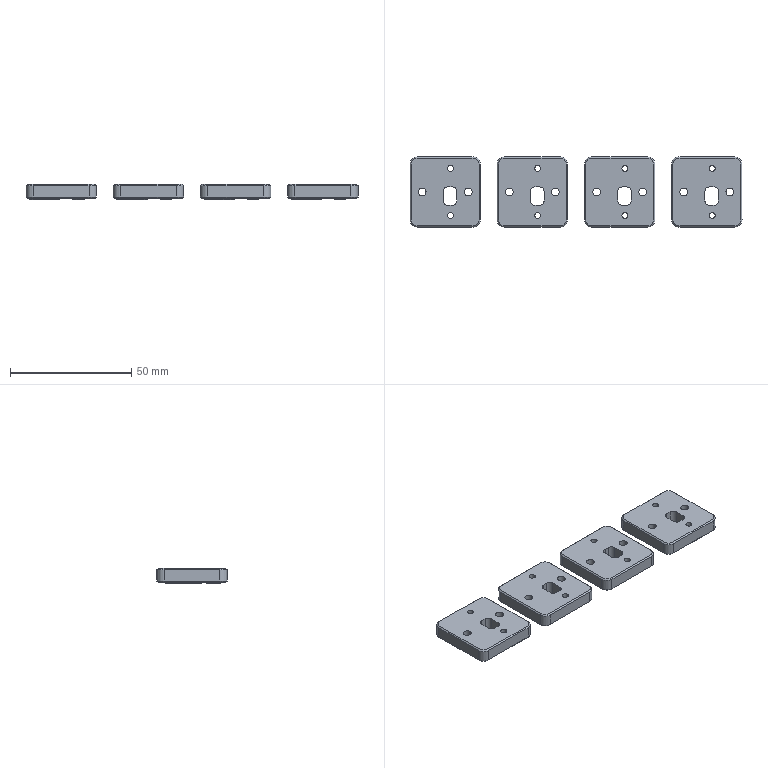NC program | NX | posted with a generic post | part box 137 x 29 x 6.3 mm
Lines 43 to 1179 of 3650:
(FLOOR_WALL_1 , TOOL : D2)
N84 T12 M6
N86 G54
N88 G17 G0 G90 X54. Y-16.497 S9500 M3
N90 G43 Z30. H12
N92 Z0.843
N94 G94 G1 Z-0.158 F1100.
N96 Y-14.497
N98 X39.503
N100 Y14.497
N102 X68.497
N104 Y-14.497
N106 X54.
N108 Y-13.497
N110 X40.503
N112 Y-10.866
N114 G3 X41.516 Y-11.2 R1.7
N116 G1 X45.516
N118 G3 X47.216 Y-9.5 R1.7
N120 G1 Y-8.5
N122 G3 X45.516 Y-6.8 R1.7
N124 G1 X41.508
N126 G3 X40.503 Y-7.134 R1.7
N128 G1 X40.622 Y-7.295
N130 G2 X41.516 Y-7. R1.5
N132 G1 X45.516
N134 G2 X47.016 Y-8.5 R1.5
N136 G1 Y-9.5
N138 G2 X45.516 Y-11. R1.5
N140 G1 X41.516
N142 G2 X40.016 Y-9.5 R1.5
N144 G1 Y-8.5
N146 G2 X40.622 Y-7.295 R1.5
N148 G1 X40.503 Y-7.134
N150 Y13.497
N152 X67.497
N154 Y-13.497
N156 X54.
N158 Y-12.497
N160 X41.503
N162 Y-12.2
N164 X45.516
N166 G3 X48.216 Y-9.5 R2.7
N168 G1 Y-8.5
N170 G3 X45.516 Y-5.8 R2.7
N172 G1 X42.503
N174 X41.503
N176 Y12.497
N178 X59.288
N180 G3 X62.317 Y12.497 R-3.2
N182 G1 X62.222 Y12.321
N184 G2 X63.445 Y8.258 R3.
N186 X62.222 Y12.321 R-3.
N188 G1 X62.317 Y12.497
N190 X66.497
N192 Y-12.497
N194 X54.
N196 Y-11.497
N198 X48.63
N200 G3 X49.216 Y-9.5 R3.7
N202 G1 Y-8.5
N204 G3 X49.206 Y-8.231 R3.7
N206 X48.3 Y-6. R-3.2
N208 G1 X48.301 Y-6.064
N210 X48.501 Y-6.06
N212 G2 X51.44 Y-3.001 R3.
N214 X48.501 Y-6.06 R-3.
N216 G1 X48.301 Y-6.064
N218 G3 X47.112 Y-5.162 R3.7
N220 G1 X47.543 Y-4.26
N222 G3 X47.726 Y-4.158 R3.45
N224 G1 X47.653 Y-4.314
N226 X47.543 Y-4.26
N228 X47.112 Y-5.162
N230 G3 X45.516 Y-4.8 R3.7
N232 G1 X42.503
N234 Y-3.632
N236 X43.503
N238 G3 X43.682 Y-3.8 R3.45
N240 G1 X43.503
N242 Y-3.632
N244 X42.503
N246 Y11.497
N248 X57.017
N250 G3 X64.588 Y11.497 R-4.2
N252 G1 X65.497
N254 Y-11.497
N256 X63.639
N258 G3 X59.364 Y-11.497 R-3.2
N260 G1 X59.498 Y-11.348
N262 G2 X59.269 Y-7.112 R3.
N264 X59.498 Y-11.348 R-3.
N266 G1 X59.364 Y-11.497
N268 X54.
N270 Y-10.497
N272 X50.109
N274 G3 X50.19 Y-9.99 R4.7
N276 X49.133 Y-2.531 R-4.2
N278 X47.248 Y1.997 R3.45
N280 X44.941 Y0.088 R1.7
N282 G2 X44.496 Y-0.45 R0.45
N284 G3 X43.557 Y-0.722 R1.7
N286 G1 X43.503 Y-0.759
N288 X43.618 Y-0.922
N290 G2 X44.494 Y-0.65 R1.5
N292 G3 X45.137 Y0.127 R0.65
N294 G2 X47.173 Y1.811 R1.5
N296 X43.221 Y-2.964 R-3.25
N298 X43.618 Y-0.922 R1.5
N300 G1 X43.503 Y-0.759
N302 Y10.497
N304 X55.667
N306 G3 X64.497 Y6.019 R5.2
N308 G1 Y-6.172
N310 G3 X57.535 Y-10.497 R4.2
N312 G1 X54.
N314 X55.349 Y-9.497
N316 G3 X50.391 Y-0.92 R5.2
N318 X50.197 Y0.128 R4.45
N320 X51.602 Y-0.614 R1.7
N322 G1 X52.7
N324 G3 X54.4 Y1.086 R1.7
N326 G1 Y3.227
N328 G3 X52.7 Y4.927 R1.7
N330 G1 X51.602
N332 G3 X49.902 Y3.227 R1.7
N334 G1 Y1.086
N336 G3 X49.926 Y0.798 R1.7
N338 G1 X50.123 Y0.832
N340 G2 X50.102 Y1.086 R1.5
N342 G1 Y3.227
N344 G2 X51.602 Y4.727 R1.5
N346 G1 X52.7
N348 G2 X54.2 Y3.227 R1.5
N350 G1 Y1.086
N352 G2 X52.7 Y-0.414 R1.5
N354 G1 X51.602
N356 G2 X50.123 Y0.832 R1.5
N358 G1 X49.926 Y0.798
N360 G3 X47.624 Y2.923 R4.45
N362 X44.503 Y2.112 R2.7
N364 G1 Y9.497
N366 X46.123
N368 G3 X45.8 Y8.5 R1.7
N370 G1 Y6.5
N372 G3 X46.716 Y4.992 R1.7
N374 G1 X46.254 Y4.105
N376 G3 X45.503 Y3.953 R3.7
N378 G1 Y4.683
N380 G3 X46.254 Y4.105 R2.7
N382 G1 X46.716 Y4.992
N384 G3 X47.5 Y4.8 R1.7
N386 G1 X48.963
N388 Y3.8
N390 G3 X48.906 Y3.379 R2.7
N392 X48.119 Y3.8 R5.45
N394 G1 X48.963
N396 Y4.8
N398 X50.5
N400 G3 X52.2 Y6.5 R1.7
N402 G1 Y8.5
N404 G3 X51.877 Y9.497 R1.7
N406 G1 X51.715 Y9.38
N408 G2 X52. Y8.5 R1.5
N410 G1 Y6.5
N412 G2 X50.5 Y5. R1.5
N414 G1 X47.5
N416 G2 X46. Y6.5 R1.5
N418 G1 Y8.5
N420 G2 X47.5 Y10. R1.5
N422 G1 X50.5
N424 G2 X51.715 Y9.38 R1.5
N426 G1 X51.877 Y9.497
N428 X54.605
N430 G3 X63.497 Y4.094 R6.2
N432 G1 Y-4.314
N434 G3 X58.135 Y-5.153 R5.2
N436 G1 X57.487 Y-4.391
N438 G3 X54.722 Y-0.703 R6.2
N440 X55.4 Y1.086 R2.7
N442 G1 Y3.227
N444 G3 X53.131 Y5.892 R2.7
N446 X53.2 Y6.5 R2.7
N448 G1 Y8.497
N450 X53.7
N452 G3 X62.497 Y2.68 R7.2
N454 G1 Y-2.996
N456 G3 X57.487 Y-4.391 R6.2
N458 G1 X57.97 Y-2.841
N460 G3 X56.072 Y-0.438 R7.2
N462 X56.272 Y0.12 R3.7
N464 X56.4 Y1.13 R3.7
N466 G1 Y2.76
N468 G3 X61.497 Y1.507 R8.2
N470 G1 Y-1.916
N472 G3 X57.97 Y-2.841 R7.2
N474 G1 X58.377 Y-1.534
N476 G3 X57.237 Y-0.141 R8.2
N478 X57.4 Y1.13 R4.7
N480 X60.497 Y0.483 R9.2
N482 G1 Y-0.978
N484 G3 X58.377 Y-1.534 R8.2
N486 G1 X58.75 Y-0.337
N488 X58.729 Y-0.309
N490 X58.796 Y-0.323
N492 X58.75 Y-0.337
N494 X57.487 Y-4.391
N496 X58.135 Y-5.153
N498 G3 X56.316 Y-9.497 R5.2
N500 G1 X55.349
N502 Y-10.497
N504 Z0.843
N506 G0 X54. Y-16.497 Z0.705
N508 G1 Z-0.295
N510 Y-14.497
N512 X39.503
N514 Y14.497
N516 X68.497
N518 Y-14.497
N520 X54.
N522 Y-13.497
N524 X40.503
N526 Y-10.866
N528 G3 X41.516 Y-11.2 R1.7
N530 G1 X45.516
N532 G3 X47.216 Y-9.5 R1.7
N534 G1 Y-8.5
N536 G3 X45.516 Y-6.8 R1.7
N538 G1 X41.508
N540 G3 X40.503 Y-7.134 R1.7
N542 G1 X40.622 Y-7.295
N544 G2 X41.516 Y-7. R1.5
N546 G1 X45.516
N548 G2 X47.016 Y-8.5 R1.5
N550 G1 Y-9.5
N552 G2 X45.516 Y-11. R1.5
N554 G1 X41.516
N556 G2 X40.016 Y-9.5 R1.5
N558 G1 Y-8.5
N560 G2 X40.622 Y-7.295 R1.5
N562 G1 X40.503 Y-7.134
N564 Y13.497
N566 X67.497
N568 Y-13.497
N570 X54.
N572 Y-12.497
N574 X41.503
N576 Y-12.2
N578 X45.516
N580 G3 X48.216 Y-9.5 R2.7
N582 G1 Y-8.5
N584 G3 X45.516 Y-5.8 R2.7
N586 G1 X42.503
N588 X41.503
N590 Y12.497
N592 X59.288
N594 G3 X62.317 Y12.497 R-3.2
N596 G1 X62.222 Y12.321
N598 G2 X63.445 Y8.258 R3.
N600 X62.222 Y12.321 R-3.
N602 G1 X62.317 Y12.497
N604 X66.497
N606 Y-12.497
N608 X54.
N610 Y-11.497
N612 X48.63
N614 G3 X49.216 Y-9.5 R3.7
N616 G1 Y-8.5
N618 G3 X49.206 Y-8.231 R3.7
N620 X48.3 Y-6. R-3.2
N622 G1 X48.301 Y-6.064
N624 X48.501 Y-6.06
N626 G2 X51.44 Y-3.001 R3.
N628 X48.501 Y-6.06 R-3.
N630 G1 X48.301 Y-6.064
N632 G3 X47.112 Y-5.162 R3.7
N634 G1 X47.543 Y-4.26
N636 G3 X47.726 Y-4.158 R3.45
N638 G1 X47.653 Y-4.314
N640 X47.543 Y-4.26
N642 X47.112 Y-5.162
N644 G3 X45.516 Y-4.8 R3.7
N646 G1 X42.503
N648 Y-3.632
N650 X43.503
N652 G3 X43.682 Y-3.8 R3.45
N654 G1 X43.503
N656 Y-3.632
N658 X42.503
N660 Y11.497
N662 X57.017
N664 G3 X64.588 Y11.497 R-4.2
N666 G1 X65.497
N668 Y-11.497
N670 X63.639
N672 G3 X59.364 Y-11.497 R-3.2
N674 G1 X59.498 Y-11.348
N676 G2 X59.269 Y-7.112 R3.
N678 X59.498 Y-11.348 R-3.
N680 G1 X59.364 Y-11.497
N682 X54.
N684 Y-10.497
N686 X50.109
N688 G3 X50.19 Y-9.99 R4.7
N690 X49.133 Y-2.531 R-4.2
N692 X47.248 Y1.997 R3.45
N694 X44.941 Y0.088 R1.7
N696 G2 X44.496 Y-0.45 R0.45
N698 G3 X43.557 Y-0.722 R1.7
N700 G1 X43.503 Y-0.759
N702 X43.618 Y-0.922
N704 G2 X44.494 Y-0.65 R1.5
N706 G3 X45.137 Y0.127 R0.65
N708 G2 X47.173 Y1.811 R1.5
N710 X43.221 Y-2.964 R-3.25
N712 X43.618 Y-0.922 R1.5
N714 G1 X43.503 Y-0.759
N716 Y10.497
N718 X55.667
N720 G3 X64.497 Y6.019 R5.2
N722 G1 Y-6.172
N724 G3 X57.535 Y-10.497 R4.2
N726 G1 X54.
N728 X55.349 Y-9.497
N730 G3 X50.391 Y-0.92 R5.2
N732 X50.197 Y0.128 R4.45
N734 X51.602 Y-0.614 R1.7
N736 G1 X52.7
N738 G3 X54.4 Y1.086 R1.7
N740 G1 Y3.227
N742 G3 X52.7 Y4.927 R1.7
N744 G1 X51.602
N746 G3 X49.902 Y3.227 R1.7
N748 G1 Y1.086
N750 G3 X49.926 Y0.798 R1.7
N752 G1 X50.123 Y0.832
N754 G2 X50.102 Y1.086 R1.5
N756 G1 Y3.227
N758 G2 X51.602 Y4.727 R1.5
N760 G1 X52.7
N762 G2 X54.2 Y3.227 R1.5
N764 G1 Y1.086
N766 G2 X52.7 Y-0.414 R1.5
N768 G1 X51.602
N770 G2 X50.123 Y0.832 R1.5
N772 G1 X49.926 Y0.798
N774 G3 X47.624 Y2.923 R4.45
N776 X44.503 Y2.112 R2.7
N778 G1 Y9.497
N780 X46.123
N782 G3 X45.8 Y8.5 R1.7
N784 G1 Y6.5
N786 G3 X46.716 Y4.992 R1.7
N788 G1 X46.254 Y4.105
N790 G3 X45.503 Y3.953 R3.7
N792 G1 Y4.683
N794 G3 X46.254 Y4.105 R2.7
N796 G1 X46.716 Y4.992
N798 G3 X47.5 Y4.8 R1.7
N800 G1 X48.963
N802 Y3.8
N804 G3 X48.906 Y3.379 R2.7
N806 X48.119 Y3.8 R5.45
N808 G1 X48.963
N810 Y4.8
N812 X50.5
N814 G3 X52.2 Y6.5 R1.7
N816 G1 Y8.5
N818 G3 X51.877 Y9.497 R1.7
N820 G1 X51.715 Y9.38
N822 G2 X52. Y8.5 R1.5
N824 G1 Y6.5
N826 G2 X50.5 Y5. R1.5
N828 G1 X47.5
N830 G2 X46. Y6.5 R1.5
N832 G1 Y8.5
N834 G2 X47.5 Y10. R1.5
N836 G1 X50.5
N838 G2 X51.715 Y9.38 R1.5
N840 G1 X51.877 Y9.497
N842 X54.605
N844 G3 X63.497 Y4.094 R6.2
N846 G1 Y-4.314
N848 G3 X58.135 Y-5.153 R5.2
N850 G1 X57.487 Y-4.391
N852 G3 X54.722 Y-0.703 R6.2
N854 X55.4 Y1.086 R2.7
N856 G1 Y3.227
N858 G3 X53.131 Y5.892 R2.7
N860 X53.2 Y6.5 R2.7
N862 G1 Y8.497
N864 X53.7
N866 G3 X62.497 Y2.68 R7.2
N868 G1 Y-2.996
N870 G3 X57.487 Y-4.391 R6.2
N872 G1 X57.97 Y-2.841
N874 G3 X56.072 Y-0.438 R7.2
N876 X56.272 Y0.12 R3.7
N878 X56.4 Y1.13 R3.7
N880 G1 Y2.76
N882 G3 X61.497 Y1.507 R8.2
N884 G1 Y-1.916
N886 G3 X57.97 Y-2.841 R7.2
N888 G1 X58.377 Y-1.534
N890 G3 X57.237 Y-0.141 R8.2
N892 X57.4 Y1.13 R4.7
N894 X60.497 Y0.483 R9.2
N896 G1 Y-0.978
N898 G3 X58.377 Y-1.534 R8.2
N900 G1 X58.75 Y-0.337
N902 X58.729 Y-0.309
N904 X58.796 Y-0.323
N906 X58.75 Y-0.337
N908 X57.487 Y-4.391
N910 X58.135 Y-5.153
N912 G3 X56.316 Y-9.497 R5.2
N914 G1 X55.349
N916 Y-10.497
N918 Z0.705
N920 G0 X54. Y-16.497 Z0.568
N922 G1 Z-0.433
N924 Y-14.497
N926 X39.503
N928 Y14.497
N930 X68.497
N932 Y-14.497
N934 X54.
N936 Y-13.497
N938 X40.503
N940 Y-10.866
N942 G3 X41.516 Y-11.2 R1.7
N944 G1 X45.516
N946 G3 X47.216 Y-9.5 R1.7
N948 G1 Y-8.5
N950 G3 X45.516 Y-6.8 R1.7
N952 G1 X41.508
N954 G3 X40.503 Y-7.134 R1.7
N956 G1 X40.622 Y-7.295
N958 G2 X41.516 Y-7. R1.5
N960 G1 X45.516
N962 G2 X47.016 Y-8.5 R1.5
N964 G1 Y-9.5
N966 G2 X45.516 Y-11. R1.5
N968 G1 X41.516
N970 G2 X40.016 Y-9.5 R1.5
N972 G1 Y-8.5
N974 G2 X40.622 Y-7.295 R1.5
N976 G1 X40.503 Y-7.134
N978 Y13.497
N980 X67.497
N982 Y-13.497
N984 X54.
N986 Y-12.497
N988 X41.503
N990 Y-12.2
N992 X45.516
N994 G3 X48.216 Y-9.5 R2.7
N996 G1 Y-8.5
N998 G3 X45.516 Y-5.8 R2.7
N1000 G1 X42.503
N1002 X41.503
N1004 Y12.497
N1006 X59.288
N1008 G3 X62.317 Y12.497 R-3.2
N1010 G1 X62.222 Y12.321
N1012 G2 X63.445 Y8.258 R3.
N1014 X62.222 Y12.321 R-3.
N1016 G1 X62.317 Y12.497
N1018 X66.497
N1020 Y-12.497
N1022 X54.
N1024 Y-11.497
N1026 X48.63
N1028 G3 X49.216 Y-9.5 R3.7
N1030 G1 Y-8.5
N1032 G3 X49.206 Y-8.231 R3.7
N1034 X48.3 Y-6. R-3.2
N1036 G1 X48.301 Y-6.064
N1038 X48.501 Y-6.06
N1040 G2 X51.44 Y-3.001 R3.
N1042 X48.501 Y-6.06 R-3.
N1044 G1 X48.301 Y-6.064
N1046 G3 X47.112 Y-5.162 R3.7
N1048 G1 X47.543 Y-4.26
N1050 G3 X47.726 Y-4.158 R3.45
N1052 G1 X47.653 Y-4.314
N1054 X47.543 Y-4.26
N1056 X47.112 Y-5.162
N1058 G3 X45.516 Y-4.8 R3.7
N1060 G1 X42.503
N1062 Y-3.632
N1064 X43.503
N1066 G3 X43.682 Y-3.8 R3.45
N1068 G1 X43.503
N1070 Y-3.632
N1072 X42.503
N1074 Y11.497
N1076 X57.017
N1078 G3 X64.588 Y11.497 R-4.2
N1080 G1 X65.497
N1082 Y-11.497
N1084 X63.639
N1086 G3 X59.364 Y-11.497 R-3.2
N1088 G1 X59.498 Y-11.348
N1090 G2 X59.269 Y-7.112 R3.
N1092 X59.498 Y-11.348 R-3.
N1094 G1 X59.364 Y-11.497
N1096 X54.
N1098 Y-10.497
N1100 X50.109
N1102 G3 X50.19 Y-9.99 R4.7
N1104 X49.133 Y-2.531 R-4.2
N1106 X47.248 Y1.997 R3.45
N1108 X44.941 Y0.088 R1.7
N1110 G2 X44.496 Y-0.45 R0.45
N1112 G3 X43.557 Y-0.722 R1.7
N1114 G1 X43.503 Y-0.759
N1116 X43.618 Y-0.922
N1118 G2 X44.494 Y-0.65 R1.5
N1120 G3 X45.137 Y0.127 R0.65
N1122 G2 X47.173 Y1.811 R1.5
N1124 X43.221 Y-2.964 R-3.25
N1126 X43.618 Y-0.922 R1.5
N1128 G1 X43.503 Y-0.759
N1130 Y10.497
N1132 X55.667
N1134 G3 X64.497 Y6.019 R5.2
N1136 G1 Y-6.172
N1138 G3 X57.535 Y-10.497 R4.2
N1140 G1 X54.
N1142 X55.349 Y-9.497
N1144 G3 X50.391 Y-0.92 R5.2
N1146 X50.197 Y0.128 R4.45
N1148 X51.602 Y-0.614 R1.7
N1150 G1 X52.7
N1152 G3 X54.4 Y1.086 R1.7
N1154 G1 Y3.227
N1156 G3 X52.7 Y4.927 R1.7
N1158 G1 X51.602
N1160 G3 X49.902 Y3.227 R1.7
N1162 G1 Y1.086
N1164 G3 X49.926 Y0.798 R1.7
N1166 G1 X50.123 Y0.832
N1168 G2 X50.102 Y1.086 R1.5
N1170 G1 Y3.227
N1172 G2 X51.602 Y4.727 R1.5
N1174 G1 X52.7
N1176 G2 X54.2 Y3.227 R1.5
N1178 G1 Y1.086
N1180 G2 X52.7 Y-0.414 R1.5
N1182 G1 X51.602
N1184 G2 X50.123 Y0.832 R1.5
N1186 G1 X49.926 Y0.798
N1188 G3 X47.624 Y2.923 R4.45
N1190 X44.503 Y2.112 R2.7
N1192 G1 Y9.497
N1194 X46.123
N1196 G3 X45.8 Y8.5 R1.7
N1198 G1 Y6.5
N1200 G3 X46.716 Y4.992 R1.7
N1202 G1 X46.254 Y4.105
N1204 G3 X45.503 Y3.953 R3.7
N1206 G1 Y4.683
N1208 G3 X46.254 Y4.105 R2.7
N1210 G1 X46.716 Y4.992
N1212 G3 X47.5 Y4.8 R1.7
N1214 G1 X48.963
N1216 Y3.8
N1218 G3 X48.906 Y3.379 R2.7
N1220 X48.119 Y3.8 R5.45
N1222 G1 X48.963
N1224 Y4.8
N1226 X50.5
N1228 G3 X52.2 Y6.5 R1.7
N1230 G1 Y8.5
N1232 G3 X51.877 Y9.497 R1.7
N1234 G1 X51.715 Y9.38
N1236 G2 X52. Y8.5 R1.5
N1238 G1 Y6.5
N1240 G2 X50.5 Y5. R1.5
N1242 G1 X47.5
N1244 G2 X46. Y6.5 R1.5
N1246 G1 Y8.5
N1248 G2 X47.5 Y10. R1.5
N1250 G1 X50.5
N1252 G2 X51.715 Y9.38 R1.5
N1254 G1 X51.877 Y9.497
N1256 X54.605
N1258 G3 X63.497 Y4.094 R6.2
N1260 G1 Y-4.314
N1262 G3 X58.135 Y-5.153 R5.2
N1264 G1 X57.487 Y-4.391
N1266 G3 X54.722 Y-0.703 R6.2
N1268 X55.4 Y1.086 R2.7
N1270 G1 Y3.227
N1272 G3 X53.131 Y5.892 R2.7
N1274 X53.2 Y6.5 R2.7
N1276 G1 Y8.497
N1278 X53.7
N1280 G3 X62.497 Y2.68 R7.2
N1282 G1 Y-2.996
N1284 G3 X57.487 Y-4.391 R6.2
N1286 G1 X57.97 Y-2.841
N1288 G3 X56.072 Y-0.438 R7.2
N1290 X56.272 Y0.12 R3.7
N1292 X56.4 Y1.13 R3.7
N1294 G1 Y2.76
N1296 G3 X61.497 Y1.507 R8.2
N1298 G1 Y-1.916
N1300 G3 X57.97 Y-2.841 R7.2
N1302 G1 X58.377 Y-1.534
N1304 G3 X57.237 Y-0.141 R8.2
N1306 X57.4 Y1.13 R4.7
N1308 X60.497 Y0.483 R9.2
N1310 G1 Y-0.978
N1312 G3 X58.377 Y-1.534 R8.2
N1314 G1 X58.75 Y-0.337
N1316 X58.729 Y-0.309
N1318 X58.796 Y-0.323
N1320 X58.75 Y-0.337
N1322 X57.487 Y-4.391
N1324 X58.135 Y-5.153
N1326 G3 X56.316 Y-9.497 R5.2
N1328 G1 X55.349
N1330 Y-10.497
N1332 Z0.568
N1334 G0 X54. Y-16.497 Z0.43
N1336 G1 Z-0.57
N1338 Y-14.497
N1340 X39.503
N1342 Y14.497
N1344 X68.497
N1346 Y-14.497
N1348 X54.
N1350 Y-13.497
N1352 X40.503
N1354 Y-10.866
N1356 G3 X41.516 Y-11.2 R1.7
N1358 G1 X45.516
N1360 G3 X47.216 Y-9.5 R1.7
N1362 G1 Y-8.5
N1364 G3 X45.516 Y-6.8 R1.7
N1366 G1 X41.508
N1368 G3 X40.503 Y-7.134 R1.7
N1370 G1 X40.622 Y-7.295
N1372 G2 X41.516 Y-7. R1.5
N1374 G1 X45.516
N1376 G2 X47.016 Y-8.5 R1.5
N1378 G1 Y-9.5
N1380 G2 X45.516 Y-11. R1.5
N1382 G1 X41.516
N1384 G2 X40.016 Y-9.5 R1.5
N1386 G1 Y-8.5
N1388 G2 X40.622 Y-7.295 R1.5
N1390 G1 X40.503 Y-7.134
N1392 Y13.497
N1394 X67.497
N1396 Y-13.497
N1398 X54.
N1400 Y-12.497
N1402 X41.503
N1404 Y-12.2
N1406 X45.516
N1408 G3 X48.216 Y-9.5 R2.7
N1410 G1 Y-8.5
N1412 G3 X45.516 Y-5.8 R2.7
N1414 G1 X42.503
N1416 X41.503
N1418 Y12.497
N1420 X59.288
N1422 G3 X62.317 Y12.497 R-3.2
N1424 G1 X62.222 Y12.321
N1426 G2 X63.445 Y8.258 R3.
N1428 X62.222 Y12.321 R-3.
N1430 G1 X62.317 Y12.497
N1432 X66.497
N1434 Y-12.497
N1436 X54.
N1438 Y-11.497
N1440 X48.63
N1442 G3 X49.216 Y-9.5 R3.7
N1444 G1 Y-8.5
N1446 G3 X49.206 Y-8.231 R3.7
N1448 X48.3 Y-6. R-3.2
N1450 G1 X48.301 Y-6.064
N1452 X48.501 Y-6.06
N1454 G2 X51.44 Y-3.001 R3.
N1456 X48.501 Y-6.06 R-3.
N1458 G1 X48.301 Y-6.064
N1460 G3 X47.112 Y-5.162 R3.7
N1462 G1 X47.543 Y-4.26
N1464 G3 X47.726 Y-4.158 R3.45
N1466 G1 X47.653 Y-4.314
N1468 X47.543 Y-4.26
N1470 X47.112 Y-5.162
N1472 G3 X45.516 Y-4.8 R3.7
N1474 G1 X42.503
N1476 Y-3.632
N1478 X43.503
N1480 G3 X43.682 Y-3.8 R3.45
N1482 G1 X43.503
N1484 Y-3.632
N1486 X42.503
N1488 Y11.497
N1490 X57.017
N1492 G3 X64.588 Y11.497 R-4.2
N1494 G1 X65.497
N1496 Y-11.497
N1498 X63.639
N1500 G3 X59.364 Y-11.497 R-3.2
N1502 G1 X59.498 Y-11.348
N1504 G2 X59.269 Y-7.112 R3.
N1506 X59.498 Y-11.348 R-3.
N1508 G1 X59.364 Y-11.497
N1510 X54.
N1512 Y-10.497
N1514 X50.109
N1516 G3 X50.19 Y-9.99 R4.7
N1518 X49.133 Y-2.531 R-4.2
N1520 X47.248 Y1.997 R3.45
N1522 X44.941 Y0.088 R1.7
N1524 G2 X44.496 Y-0.45 R0.45
N1526 G3 X43.557 Y-0.722 R1.7
N1528 G1 X43.503 Y-0.759
N1530 X43.618 Y-0.922
N1532 G2 X44.494 Y-0.65 R1.5
N1534 G3 X45.137 Y0.127 R0.65
N1536 G2 X47.173 Y1.811 R1.5
N1538 X43.221 Y-2.964 R-3.25
N1540 X43.618 Y-0.922 R1.5
N1542 G1 X43.503 Y-0.759
N1544 Y10.497
N1546 X55.667
N1548 G3 X64.497 Y6.019 R5.2
N1550 G1 Y-6.172
N1552 G3 X57.535 Y-10.497 R4.2
N1554 G1 X54.
N1556 X55.349 Y-9.497
N1558 G3 X50.391 Y-0.92 R5.2
N1560 X50.197 Y0.128 R4.45
N1562 X51.602 Y-0.614 R1.7
N1564 G1 X52.7
N1566 G3 X54.4 Y1.086 R1.7
N1568 G1 Y3.227
N1570 G3 X52.7 Y4.927 R1.7
N1572 G1 X51.602
N1574 G3 X49.902 Y3.227 R1.7
N1576 G1 Y1.086
N1578 G3 X49.926 Y0.798 R1.7
N1580 G1 X50.123 Y0.832
N1582 G2 X50.102 Y1.086 R1.5
N1584 G1 Y3.227
N1586 G2 X51.602 Y4.727 R1.5
N1588 G1 X52.7
N1590 G2 X54.2 Y3.227 R1.5
N1592 G1 Y1.086
N1594 G2 X52.7 Y-0.414 R1.5
N1596 G1 X51.602
N1598 G2 X50.123 Y0.832 R1.5
N1600 G1 X49.926 Y0.798
N1602 G3 X47.624 Y2.923 R4.45
N1604 X44.503 Y2.112 R2.7
N1606 G1 Y9.497
N1608 X46.123
N1610 G3 X45.8 Y8.5 R1.7
N1612 G1 Y6.5
N1614 G3 X46.716 Y4.992 R1.7
N1616 G1 X46.254 Y4.105
N1618 G3 X45.503 Y3.953 R3.7
N1620 G1 Y4.683
N1622 G3 X46.254 Y4.105 R2.7
N1624 G1 X46.716 Y4.992
N1626 G3 X47.5 Y4.8 R1.7
N1628 G1 X48.963
N1630 Y3.8
N1632 G3 X48.906 Y3.379 R2.7
N1634 X48.119 Y3.8 R5.45
N1636 G1 X48.963
N1638 Y4.8
N1640 X50.5
N1642 G3 X52.2 Y6.5 R1.7
N1644 G1 Y8.5
N1646 G3 X51.877 Y9.497 R1.7
N1648 G1 X51.715 Y9.38
N1650 G2 X52. Y8.5 R1.5
N1652 G1 Y6.5
N1654 G2 X50.5 Y5. R1.5
N1656 G1 X47.5
N1658 G2 X46. Y6.5 R1.5
N1660 G1 Y8.5
N1662 G2 X47.5 Y10. R1.5
N1664 G1 X50.5
N1666 G2 X51.715 Y9.38 R1.5
N1668 G1 X51.877 Y9.497
N1670 X54.605
N1672 G3 X63.497 Y4.094 R6.2
N1674 G1 Y-4.314
N1676 G3 X58.135 Y-5.153 R5.2
N1678 G1 X57.487 Y-4.391
N1680 G3 X54.722 Y-0.703 R6.2
N1682 X55.4 Y1.086 R2.7
N1684 G1 Y3.227
N1686 G3 X53.131 Y5.892 R2.7
N1688 X53.2 Y6.5 R2.7
N1690 G1 Y8.497
N1692 X53.7
N1694 G3 X62.497 Y2.68 R7.2
N1696 G1 Y-2.996
N1698 G3 X57.487 Y-4.391 R6.2
N1700 G1 X57.97 Y-2.841
N1702 G3 X56.072 Y-0.438 R7.2
N1704 X56.272 Y0.12 R3.7
N1706 X56.4 Y1.13 R3.7
N1708 G1 Y2.76
N1710 G3 X61.497 Y1.507 R8.2
N1712 G1 Y-1.916
N1714 G3 X57.97 Y-2.841 R7.2
N1716 G1 X58.377 Y-1.534
N1718 G3 X57.237 Y-0.141 R8.2
N1720 X57.4 Y1.13 R4.7
N1722 X60.497 Y0.483 R9.2
N1724 G1 Y-0.978
N1726 G3 X58.377 Y-1.534 R8.2
N1728 G1 X58.75 Y-0.337
N1730 X58.729 Y-0.309
N1732 X58.796 Y-0.323
N1734 X58.75 Y-0.337
N1736 X57.487 Y-4.391
N1738 X58.135 Y-5.153
N1740 G3 X56.316 Y-9.497 R5.2
N1742 G1 X55.349
N1744 Y-10.497
N1746 Z0.43
N1748 G0 Z30.
N1750 X18. Y-16.497
N1752 Z0.843
N1754 G1 Z-0.158
N1756 Y-14.497
N1758 X3.503
N1760 Y14.497
N1762 X32.497
N1764 Y-14.497
N1766 X18.
N1768 Y-13.497
N1770 X4.503
N1772 Y-10.866
N1774 G3 X5.516 Y-11.2 R1.7
N1776 G1 X9.516
N1778 G3 X11.216 Y-9.5 R1.7
N1780 G1 Y-8.5
N1782 G3 X9.516 Y-6.8 R1.7
N1784 G1 X5.508
N1786 G3 X4.503 Y-7.134 R1.7
N1788 G1 X4.622 Y-7.295
N1790 G2 X5.516 Y-7. R1.5
N1792 G1 X9.516
N1794 G2 X11.016 Y-8.5 R1.5
N1796 G1 Y-9.5
N1798 G2 X9.516 Y-11. R1.5
N1800 G1 X5.516
N1802 G2 X4.016 Y-9.5 R1.5
N1804 G1 Y-8.5
N1806 G2 X4.622 Y-7.295 R1.5
N1808 G1 X4.503 Y-7.134
N1810 Y13.497
N1812 X31.497
N1814 Y-13.497
N1816 X18.
N1818 Y-12.497
N1820 X5.503
N1822 Y-12.2
N1824 X9.516
N1826 G3 X12.216 Y-9.5 R2.7
N1828 G1 Y-8.5
N1830 G3 X9.516 Y-5.8 R2.7
N1832 G1 X5.503
N1834 Y12.497
N1836 X23.288
N1838 G3 X26.317 Y12.497 R-3.2
N1840 G1 X26.222 Y12.321
N1842 G2 X27.445 Y8.258 R3.
N1844 X26.222 Y12.321 R-3.
N1846 G1 X26.317 Y12.497
N1848 X30.497
N1850 Y-12.497
N1852 X18.
N1854 Y-11.497
N1856 X12.63
N1858 G3 X13.216 Y-9.5 R3.7
N1860 G1 Y-8.5
N1862 G3 X13.206 Y-8.231 R3.7
N1864 X12.3 Y-6. R-3.2
N1866 G1 X12.301 Y-6.064
N1868 X12.501 Y-6.06
N1870 G2 X15.44 Y-3.001 R3.
N1872 X12.501 Y-6.06 R-3.
N1874 G1 X12.301 Y-6.064
N1876 G3 X11.112 Y-5.162 R3.7
N1878 G1 X11.543 Y-4.26
N1880 G3 X11.726 Y-4.158 R3.45
N1882 G1 X11.653 Y-4.314
N1884 X11.543 Y-4.26
N1886 X11.112 Y-5.162
N1888 G3 X9.516 Y-4.8 R3.7
N1890 G1 X6.503
N1892 Y-3.632
N1894 X7.503
N1896 G3 X7.682 Y-3.8 R3.45
N1898 G1 X7.503
N1900 Y-3.632
N1902 X6.503
N1904 Y11.497
N1906 X21.017
N1908 G3 X28.588 Y11.497 R-4.2
N1910 G1 X29.497
N1912 Y-11.497
N1914 X27.639
N1916 G3 X23.364 Y-11.497 R-3.2
N1918 G1 X23.498 Y-11.348
N1920 G2 X23.269 Y-7.112 R3.
N1922 X23.498 Y-11.348 R-3.
N1924 G1 X23.364 Y-11.497
N1926 X18.
N1928 Y-10.497
N1930 X14.109
N1932 G3 X14.19 Y-9.99 R4.7
N1934 X13.133 Y-2.531 R-4.2
N1936 X11.248 Y1.997 R3.45
N1938 X8.941 Y0.088 R1.7
N1940 G2 X8.496 Y-0.45 R0.45
N1942 G3 X7.557 Y-0.722 R1.7
N1944 G1 X7.503 Y-0.759
N1946 X7.618 Y-0.922
N1948 G2 X8.494 Y-0.65 R1.5
N1950 G3 X9.137 Y0.127 R0.65
N1952 G2 X11.173 Y1.811 R1.5
N1954 X7.221 Y-2.964 R-3.25
N1956 X7.618 Y-0.922 R1.5
N1958 G1 X7.503 Y-0.759
N1960 Y10.497
N1962 X19.667
N1964 G3 X28.497 Y6.019 R5.2
N1966 G1 Y-6.172
N1968 G3 X21.535 Y-10.497 R4.2
N1970 G1 X18.
N1972 X19.349 Y-9.497
N1974 G3 X14.391 Y-0.92 R5.2
N1976 X14.197 Y0.128 R4.45
N1978 X15.602 Y-0.614 R1.7
N1980 G1 X16.7
N1982 G3 X18.4 Y1.086 R1.7
N1984 G1 Y3.227
N1986 G3 X16.7 Y4.927 R1.7
N1988 G1 X15.602
N1990 G3 X13.902 Y3.227 R1.7
N1992 G1 Y1.086
N1994 G3 X13.926 Y0.798 R1.7
N1996 G1 X14.123 Y0.832
N1998 G2 X14.102 Y1.086 R1.5
N2000 G1 Y3.227
N2002 G2 X15.602 Y4.727 R1.5
N2004 G1 X16.7
N2006 G2 X18.2 Y3.227 R1.5
N2008 G1 Y1.086
N2010 G2 X16.7 Y-0.414 R1.5
N2012 G1 X15.602
N2014 G2 X14.123 Y0.832 R1.5
N2016 G1 X13.926 Y0.798
N2018 G3 X11.624 Y2.923 R4.45
N2020 X8.503 Y2.112 R2.7
N2022 G1 Y9.497
N2024 X10.123
N2026 G3 X9.8 Y8.5 R1.7
N2028 G1 Y6.5
N2030 G3 X10.716 Y4.992 R1.7
N2032 G1 X10.254 Y4.105
N2034 G3 X9.503 Y3.953 R3.7
N2036 G1 Y4.683
N2038 G3 X10.254 Y4.105 R2.7
N2040 G1 X10.716 Y4.992
N2042 G3 X11.5 Y4.8 R1.7
N2044 G1 X12.963
N2046 Y3.8
N2048 G3 X12.906 Y3.379 R2.7
N2050 X12.119 Y3.8 R5.45
N2052 G1 X12.963
N2054 Y4.8
N2056 X14.5
N2058 G3 X16.2 Y6.5 R1.7
N2060 G1 Y8.5
N2062 G3 X15.877 Y9.497 R1.7
N2064 G1 X15.715 Y9.38
N2066 G2 X16. Y8.5 R1.5
N2068 G1 Y6.5
N2070 G2 X14.5 Y5. R1.5
N2072 G1 X11.5
N2074 G2 X10. Y6.5 R1.5
N2076 G1 Y8.5
N2078 G2 X11.5 Y10. R1.5
N2080 G1 X14.5
N2082 G2 X15.715 Y9.38 R1.5
N2084 G1 X15.877 Y9.497
N2086 X18.605
N2088 G3 X27.497 Y4.094 R6.2
N2090 G1 Y-4.314
N2092 G3 X22.135 Y-5.153 R5.2
N2094 G1 X21.487 Y-4.391
N2096 G3 X18.722 Y-0.703 R6.2
N2098 X19.4 Y1.086 R2.7
N2100 G1 Y3.227
N2102 G3 X17.131 Y5.892 R2.7
N2104 X17.2 Y6.5 R2.7
N2106 G1 Y8.497
N2108 X17.7
N2110 G3 X26.497 Y2.68 R7.2
N2112 G1 Y-2.996
N2114 G3 X21.487 Y-4.391 R6.2
N2116 G1 X21.97 Y-2.841
N2118 G3 X20.072 Y-0.438 R7.2
N2120 X20.272 Y0.12 R3.7
N2122 X20.4 Y1.13 R3.7
N2124 G1 Y2.76
N2126 G3 X25.497 Y1.507 R8.2
N2128 G1 Y-1.916
N2130 G3 X21.97 Y-2.841 R7.2
N2132 G1 X22.377 Y-1.534
N2134 G3 X21.237 Y-0.141 R8.2
N2136 X21.4 Y1.13 R4.7
N2138 X24.497 Y0.483 R9.2
N2140 G1 Y-0.978
N2142 G3 X22.377 Y-1.534 R8.2
N2144 G1 X22.75 Y-0.337
N2146 X22.729 Y-0.309
N2148 X22.796 Y-0.323
N2150 X22.75 Y-0.337
N2152 X21.487 Y-4.391
N2154 X22.135 Y-5.153
N2156 G3 X20.316 Y-9.497 R5.2
N2158 G1 X19.349
N2160 Y-10.497
N2162 Z0.843
N2164 G0 X18. Y-16.497 Z0.705
N2166 G1 Z-0.295
N2168 Y-14.497
N2170 X3.503
N2172 Y14.497
N2174 X32.497
N2176 Y-14.497
N2178 X18.
N2180 Y-13.497
N2182 X4.503
N2184 Y-10.866
N2186 G3 X5.516 Y-11.2 R1.7
N2188 G1 X9.516
N2190 G3 X11.216 Y-9.5 R1.7
N2192 G1 Y-8.5
N2194 G3 X9.516 Y-6.8 R1.7
N2196 G1 X5.508
N2198 G3 X4.503 Y-7.134 R1.7
N2200 G1 X4.622 Y-7.295
N2202 G2 X5.516 Y-7. R1.5
N2204 G1 X9.516
N2206 G2 X11.016 Y-8.5 R1.5
N2208 G1 Y-9.5
N2210 G2 X9.516 Y-11. R1.5
N2212 G1 X5.516
N2214 G2 X4.016 Y-9.5 R1.5
N2216 G1 Y-8.5
N2218 G2 X4.622 Y-7.295 R1.5
N2220 G1 X4.503 Y-7.134
N2222 Y13.497
N2224 X31.497
N2226 Y-13.497
N2228 X18.
N2230 Y-12.497
N2232 X5.503
N2234 Y-12.2
N2236 X9.516
N2238 G3 X12.216 Y-9.5 R2.7
N2240 G1 Y-8.5
N2242 G3 X9.516 Y-5.8 R2.7
N2244 G1 X5.503
N2246 Y12.497
N2248 X23.288
N2250 G3 X26.317 Y12.497 R-3.2
N2252 G1 X26.222 Y12.321
N2254 G2 X27.445 Y8.258 R3.
N2256 X26.222 Y12.321 R-3.
N2258 G1 X26.317 Y12.497
N2260 X30.497
N2262 Y-12.497
N2264 X18.
N2266 Y-11.497
N2268 X12.63
N2270 G3 X13.216 Y-9.5 R3.7
N2272 G1 Y-8.5
N2274 G3 X13.206 Y-8.231 R3.7
N2276 X12.3 Y-6. R-3.2
N2278 G1 X12.301 Y-6.064
N2280 X12.501 Y-6.06
N2282 G2 X15.44 Y-3.001 R3.
N2284 X12.501 Y-6.06 R-3.
N2286 G1 X12.301 Y-6.064
N2288 G3 X11.112 Y-5.162 R3.7
N2290 G1 X11.543 Y-4.26
N2292 G3 X11.726 Y-4.158 R3.45
N2294 G1 X11.653 Y-4.314
N2296 X11.543 Y-4.26
N2298 X11.112 Y-5.162
N2300 G3 X9.516 Y-4.8 R3.7
N2302 G1 X6.503
N2304 Y-3.632
N2306 X7.503
N2308 G3 X7.682 Y-3.8 R3.45
N2310 G1 X7.503
N2312 Y-3.632
N2314 X6.503
N2316 Y11.497
N2318 X21.017
N2320 G3 X28.588 Y11.497 R-4.2
N2322 G1 X29.497
N2324 Y-11.497
N2326 X27.639
N2328 G3 X23.364 Y-11.497 R-3.2
N2330 G1 X23.498 Y-11.348
N2332 G2 X23.269 Y-7.112 R3.
N2334 X23.498 Y-11.348 R-3.
N2336 G1 X23.364 Y-11.497
N2338 X18.
N2340 Y-10.497
N2342 X14.109
N2344 G3 X14.19 Y-9.99 R4.7
N2346 X13.133 Y-2.531 R-4.2
N2348 X11.248 Y1.997 R3.45
N2350 X8.941 Y0.088 R1.7